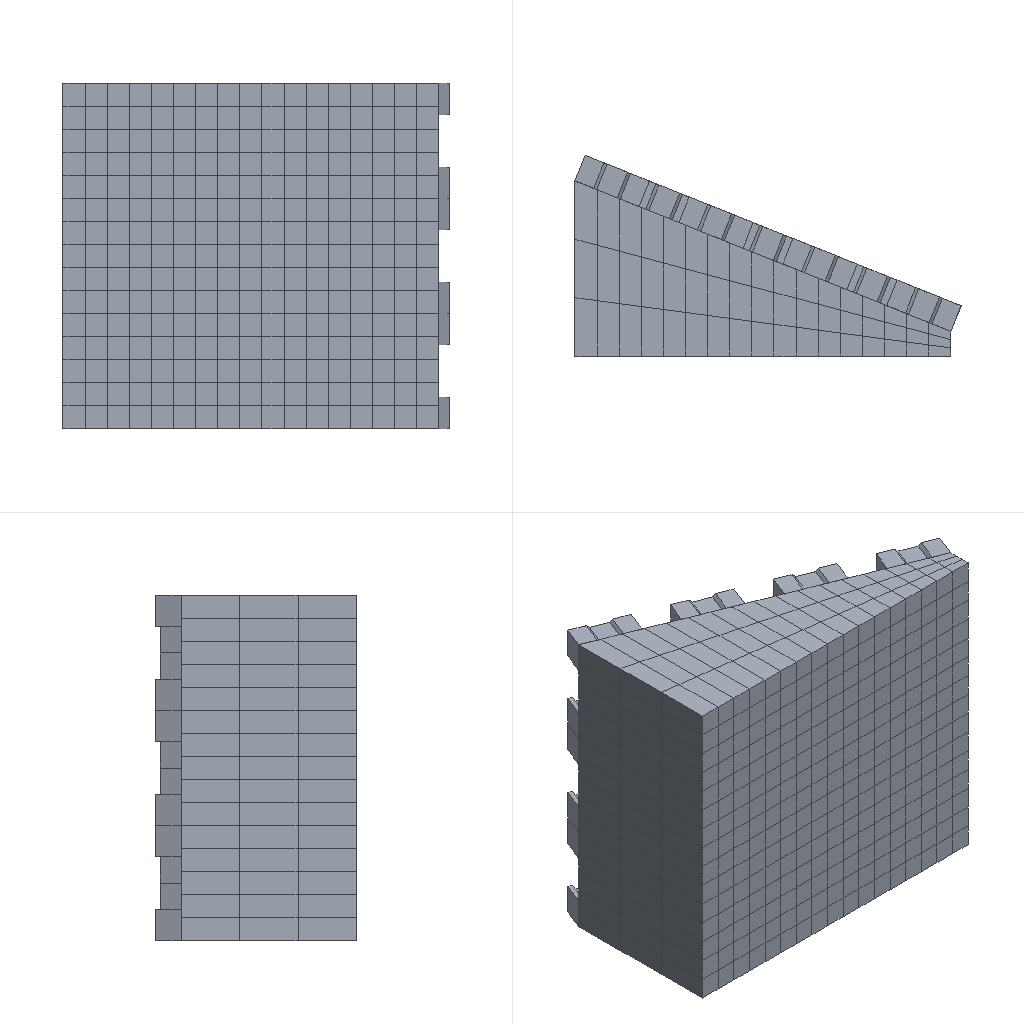Simulation study | abaqus
Set-up summary:
category,name,step,type,value,unit,region
solver,abaqus
solver,version,,,Abaqus/Standard 2020
units,not stated in the deck,,not stated
analysis,deck,,geostatic,geostatic; transient
load_step,Step-1,Step-1,geostatic,nlgeom=True
load_step,Step-2,Step-2,transient,nlgeom=True
contact,interactions,,,general=1 pairs=1 ties=0
load_step,requested,,,2
mesh,nodes,,,3816
mesh,elements,,,1809
element_type,C3D8R,,solid,1809
load,load commands in deck,,count,2
bc,support commands in deck,,count,9
material,HUNNINGTU,,in results
material,SOIL,,in results
check,setup vs results,,match,"per instance, exact: element labels, types and connectivity; labels of the nodes the elements use; coordinates of those nodes at SINGLE_PRECISION in 3 of 19 instance(s)"
Results summary:
result,step,,completed,increments=11 time=1.0/1.0
result,step,,completed,increments=25 time=1.0/1.0
result,analysis,,,transient
result,last_loadstep,,,2
result,analysis steps,,count,2
result,primary field,,,U
result,reaction total,,FX,-24113322.655,model units
result,reaction total,,FY,26337993866.0,model units
result,reaction total,,FZ,-87043.066,model units